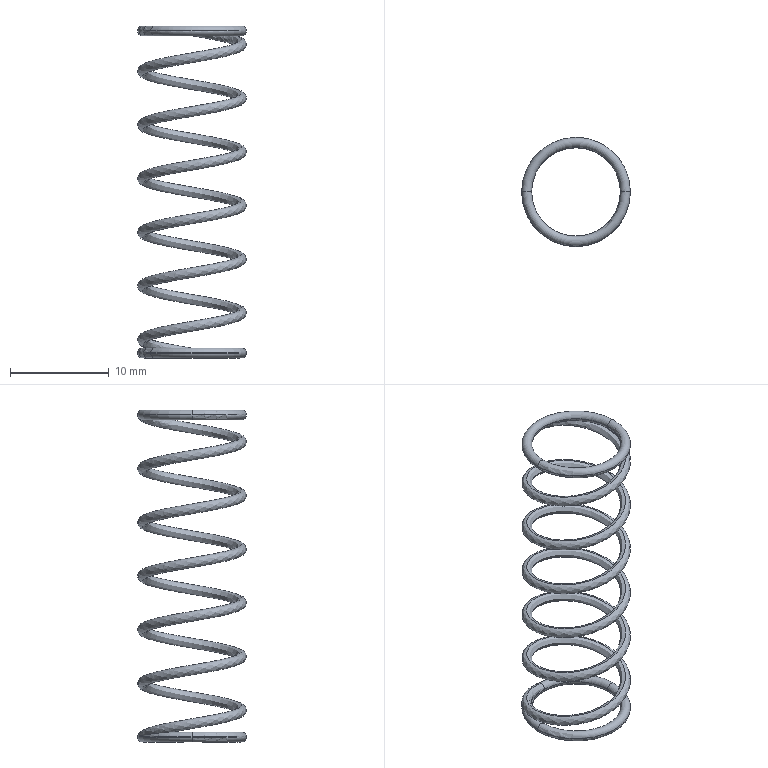Part | STEP file | 8xs282020 | 1 solid | 16 faces | box 11 x 11 x 33.6 mm | volume 193.342 mm3 | torus 10 | cylinder 2 | spline 2 | plane 2 | commonest cylinder face diameters 10.12 x2